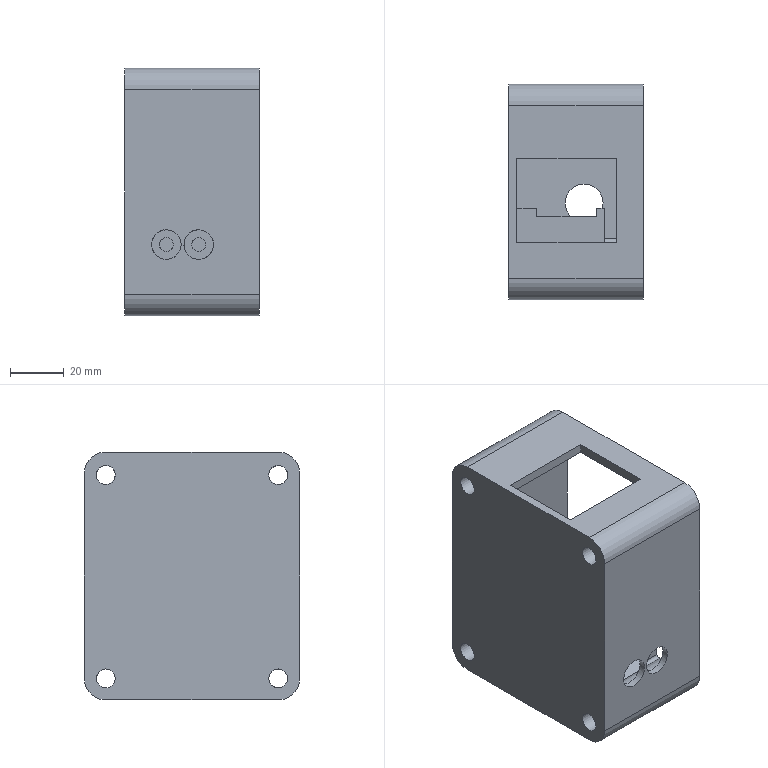NC program | NX | posted by the shop | part box 50 x 80 x 92 mm
Whole program:
%
O1234(3)
(T=7 D6-18-D6-50-3T-rough Z=-18.00 D=6.00 R=0.00 L=50.00)
()
(T=0 Drill D5.1-62-92 Z=-62.00 D=5.10 R=0.00 L=92.00)
G40 G17 G80 G90 G21
M9
M5
G91 G28 Z0.0
M1
N1
(T=11 N=D6-18-D6-50-3T-rough D=1.00 R=0.00 FL=10.00 L=11.00)
(XY-STOCK=0.05)
T11 M6
T2
G0 G90 G54 X-19.5 Y-15.5 S4000 M3
G43 H11 Z20.
M8
Z.5
G3 Y-17.95 I0.0 J-1.225 F800.
X-19.5 Y-17.95 Z.3 I0.0 J2.45
X-19.5 Y-17.95 Z.1 I0.0 J2.45
X-19.5 Y-17.95 Z-.1 I0.0 J2.45
X-19.5 Y-17.95 Z-.3 I0.0 J2.45
X-19.5 Y-17.95 Z-.5 I0.0 J2.45
X-19.5 Y-17.95 Z-.7 I0.0 J2.45
X-19.5 Y-17.95 Z-.9 I0.0 J2.45
X-19.5 Y-17.95 Z-1.1 I0.0 J2.45
X-19.5 Y-17.95 Z-1.3 I0.0 J2.45
X-19.5 Y-17.95 Z-1.5 I0.0 J2.45
X-19.5 Y-17.95 Z-1.7 I0.0 J2.45
X-19.5 Y-17.95 Z-1.9 I0.0 J2.45
X-19.5 Y-17.95 Z-2.1 I0.0 J2.45
X-19.5 Y-17.95 Z-2.3 I0.0 J2.45
X-19.5 Y-17.95 Z-2.5 I0.0 J2.45
X-19.5 Y-17.95 Z-2.7 I0.0 J2.45
X-19.5 Y-17.95 Z-2.9 I0.0 J2.45
X-19.5 Y-13.05 Z-3. I0.0 J2.45
I0.0 J-2.45
Y-15.5 I0.0 J-1.225
G0 Z20.
Y-27.5
Z.5
G3 Y-29.95 I0.0 J-1.225
X-19.5 Y-29.95 Z.3 I0.0 J2.45
X-19.5 Y-29.95 Z.1 I0.0 J2.45
X-19.5 Y-29.95 Z-.1 I0.0 J2.45
X-19.5 Y-29.95 Z-.3 I0.0 J2.45
X-19.5 Y-29.95 Z-.5 I0.0 J2.45
X-19.5 Y-29.95 Z-.7 I0.0 J2.45
X-19.5 Y-29.95 Z-.9 I0.0 J2.45
X-19.5 Y-29.95 Z-1.1 I0.0 J2.45
X-19.5 Y-29.95 Z-1.3 I0.0 J2.45
X-19.5 Y-29.95 Z-1.5 I0.0 J2.45
X-19.5 Y-29.95 Z-1.7 I0.0 J2.45
X-19.5 Y-29.95 Z-1.9 I0.0 J2.45
X-19.5 Y-29.95 Z-2.1 I0.0 J2.45
X-19.5 Y-29.95 Z-2.3 I0.0 J2.45
X-19.5 Y-29.95 Z-2.5 I0.0 J2.45
X-19.5 Y-29.95 Z-2.7 I0.0 J2.45
X-19.5 Y-29.95 Z-2.9 I0.0 J2.45
X-19.5 Y-25.05 Z-3. I0.0 J2.45
I0.0 J-2.45
Y-27.5 I0.0 J-1.225
G0 Z20.
G0 X-19.5 Y-15.5 S4000 M3
M8
Z-3.
G3 Y-18. I0.0 J-1.25 F800.
I0.0 J2.5
Y-15.5 I0.0 J1.25
G0 Z20.
Y-27.5
Z-3.
G3 Y-30. I0.0 J-1.25
I0.0 J2.5
Y-27.5 I0.0 J1.25
G0 Z20.
M9
M5
G91 G28 Z0.0
M1
N2
(T=2 N=点孔D8-120-90度 D=8.00 R=0.00 FL=0.00 L=120.00)
(XY-STOCK=0.00)
T2 M6
T16
G0 G90 G54 X-19.5 Y-15.5 S2000 M3
G43 H02 Z20.
M8
G98 G81 X-19.5 Y-15.5 Z-17.9 R-12. F200.
Y-27.5
G80
G0 X-19.5 Y-27.5 Z20.
M9
M5
G91 G28 Z0.0
M1
N3
(T=16 N=Drill D5.1-62-92 D=5.10 R=0.00 FL=62.00 L=92.00)
(XY-STOCK=0.00)
T16 M6
T11
G0 G90 G54 X-19.5 Y-15.5 S2000 M3
G43 H16 Z20.
M8
G98 G83 X-19.5 Y-15.5 Z-35. R-12. F200. Q2.
Y-27.5
G80
G0 X-19.5 Y-27.5 Z20.
M9
M5
G91 G28 Z0.0
G28 Y0.
M30
%